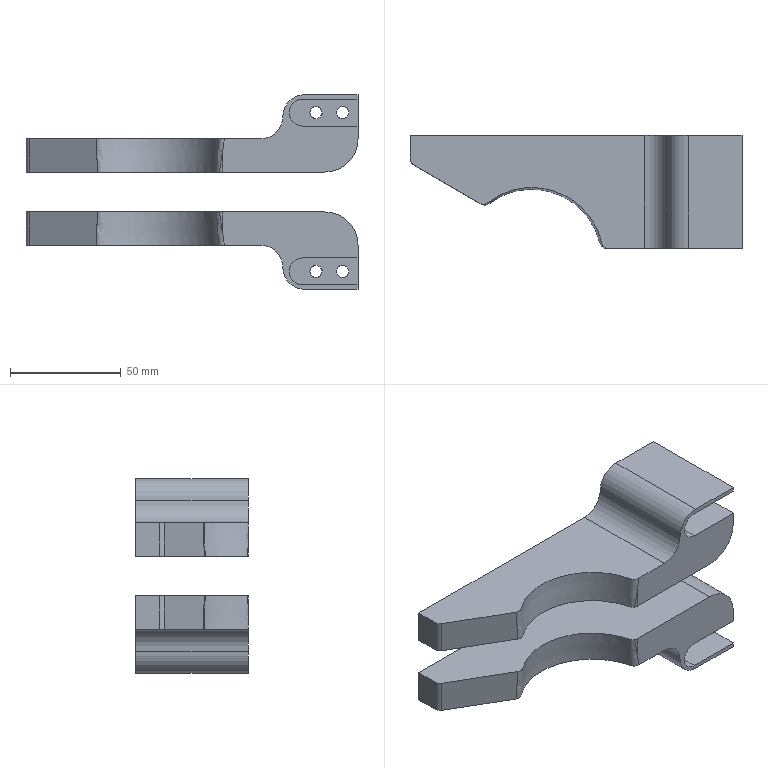NC program | NX | posted with a generic post | part box 150 x 51 x 88 mm
Lines 8852 to 9163 of 21230:
(ZLEVEL_PROFILE_COPY_COPY_COPY_1_COPY_COPY_COPY_COPY , TOOL : D12JING)
N17678 T11 M6
N17680 G54
N17682 G17 G0 G90 X-77.567 Y26.742 S9500 M3
N17684 G43 Z30. H11
N17686 Z-8.5
N17688 G94 G1 X-76.038 Y24.095 F1000.
N17690 G3 X-75. Y23.495 R1.199
N17692 G1 X60.005 F1200.
N17694 G2 X80.995 Y2.5 R20.995
N17696 G1 Y-17.5
N17698 G2 X75. Y-23.495 R5.995
N17700 G1 X51.
N17702 G2 X35.005 Y-7.5 R15.995
N17704 G3 X31. Y-3.495 R4.005
N17706 G1 X-75.
N17708 G2 X-80.995 Y2.5 R5.995
N17710 G1 Y17.5
N17712 G2 X-75. Y23.495 R5.995
N17714 G3 X-73.962 Y24.095 R1.199
N17716 G1 X-72.231 Y27.092
N17718 G0 X-77.567 Y26.742 Z-17.
N17720 G1 X-76.038 Y24.095 F1000.
N17722 G3 X-75. Y23.495 R1.199
N17724 G1 X60.005 F1200.
N17726 G2 X80.995 Y2.5 R20.995
N17728 G1 Y-17.5
N17730 G2 X75. Y-23.495 R5.995
N17732 G1 X51.
N17734 G2 X35.005 Y-7.5 R15.995
N17736 G3 X31. Y-3.495 R4.005
N17738 G1 X-75.
N17740 G2 X-80.995 Y2.5 R5.995
N17742 G1 Y17.5
N17744 G2 X-75. Y23.495 R5.995
N17746 G3 X-73.962 Y24.095 R1.199
N17748 G1 X-72.231 Y27.092
N17750 G0 X-77.567 Y26.742 Z-25.5
N17752 G1 X-76.038 Y24.095 F1000.
N17754 G3 X-75. Y23.495 R1.199
N17756 G1 X60.005 F1200.
N17758 G2 X80.995 Y2.5 R20.995
N17760 G1 Y-17.5
N17762 G2 X75. Y-23.495 R5.995
N17764 G1 X51.
N17766 G2 X35.005 Y-7.5 R15.995
N17768 G3 X31. Y-3.495 R4.005
N17770 G1 X-75.
N17772 G2 X-80.995 Y2.5 R5.995
N17774 G1 Y17.5
N17776 G2 X-75. Y23.495 R5.995
N17778 G3 X-73.962 Y24.095 R1.199
N17780 G1 X-72.231 Y27.092
N17782 G0 X-77.567 Y26.742 Z-34.
N17784 G1 X-76.038 Y24.095 F1000.
N17786 G3 X-75. Y23.495 R1.199
N17788 G1 X60.005 F1200.
N17790 G2 X80.995 Y2.5 R20.995
N17792 G1 Y-17.5
N17794 G2 X75. Y-23.495 R5.995
N17796 G1 X51.
N17798 G2 X35.005 Y-7.5 R15.995
N17800 G3 X31. Y-3.495 R4.005
N17802 G1 X-75.
N17804 G2 X-80.995 Y2.5 R5.995
N17806 G1 Y17.5
N17808 G2 X-75. Y23.495 R5.995
N17810 G3 X-73.962 Y24.095 R1.199
N17812 G1 X-72.231 Y27.092
N17814 G0 X-77.567 Y26.742 Z-42.5
N17816 G1 X-76.038 Y24.095 F1000.
N17818 G3 X-75. Y23.495 R1.199
N17820 G1 X60.005 F1200.
N17822 G2 X80.995 Y2.5 R20.995
N17824 G1 Y-17.5
N17826 G2 X75. Y-23.495 R5.995
N17828 G1 X51.
N17830 G2 X35.005 Y-7.5 R15.995
N17832 G3 X31. Y-3.495 R4.005
N17834 G1 X-75.
N17836 G2 X-80.995 Y2.5 R5.995
N17838 G1 Y17.5
N17840 G2 X-75. Y23.495 R5.995
N17842 G3 X-73.962 Y24.095 R1.199
N17844 G1 X-72.231 Y27.092
N17846 G0 X-77.567 Y26.742 Z-51.
N17848 G1 X-76.038 Y24.095 F1000.
N17850 G3 X-75. Y23.495 R1.199
N17852 G1 X60.005 F1200.
N17854 G2 X80.995 Y2.5 R20.995
N17856 G1 Y-17.5
N17858 G2 X75. Y-23.495 R5.995
N17860 G1 X51.
N17862 G2 X35.005 Y-7.5 R15.995
N17864 G3 X31. Y-3.495 R4.005
N17866 G1 X-75.
N17868 G2 X-80.995 Y2.5 R5.995
N17870 G1 Y17.5
N17872 G2 X-75. Y23.495 R5.995
N17874 G3 X-73.962 Y24.095 R1.199
N17876 G1 X-72.231 Y27.092
N17878 G0 Z30.
(ZLEVEL_PROFILE_COPY , TOOL : D12JING)
N17880 X81.455 Y-9.292
N17882 Z0.
N17884 G1 Z-0.95 F1650.
N17886 X80.966 Y-9.295
N17888 X74.609
N17890 X50.
N17892 G3 X49.895 Y-9.4 R0.105
N17894 X50. Y-9.505 R0.105
N17896 G1 X74.609
N17898 X80.966
N17900 X81.455 Y-9.507
N17902 G3 X81.755 Y-9.429 R0.6
N17904 G0 X81.455 Y-9.292
N17906 G1 Z-1.9
N17908 X80.966 Y-9.296
N17910 X74.609 Y-9.295
N17912 X50.
N17914 G3 X49.895 Y-9.4 R0.105
N17916 X50. Y-9.505 R0.105
N17918 G1 X74.609
N17920 X80.966 Y-9.504
N17922 X81.455 Y-9.507
N17924 G3 X81.755 Y-9.429 R0.6
N17926 G0 X81.455 Y-9.292
N17928 G1 Z-2.85
N17930 X80.966 Y-9.296
N17932 X74.609 Y-9.295
N17934 X50.
N17936 G3 X49.895 Y-9.4 R0.105
N17938 X50. Y-9.505 R0.105
N17940 G1 X74.609
N17942 X80.966 Y-9.504
N17944 X81.455 Y-9.507
N17946 G3 X81.755 Y-9.429 R0.6
N17948 G0 X81.455 Y-9.292
N17950 G1 Z-3.8
N17952 X80.966 Y-9.296
N17954 X75.098
N17956 X74.609 Y-9.295
N17958 X50.
N17960 G3 X49.895 Y-9.4 R0.105
N17962 X50. Y-9.505 R0.105
N17964 G1 X74.609
N17966 X75.098 Y-9.504
N17968 X80.966
N17970 X81.455 Y-9.507
N17972 G3 X81.755 Y-9.428 R0.6
N17974 G0 X81.455 Y-9.292
N17976 G1 Z-4.75
N17978 X80.966 Y-9.296
N17980 X75.098
N17982 X74.609 Y-9.295
N17984 X50.
N17986 G3 X49.895 Y-9.4 R0.105
N17988 X50. Y-9.505 R0.105
N17990 G1 X74.609
N17992 X75.098 Y-9.504
N17994 X80.966
N17996 X81.455 Y-9.507
N17998 G3 X81.755 Y-9.428 R0.6
N18000 G0 X81.455 Y-9.292
N18002 G1 Z-5.7
N18004 X80.966 Y-9.296
N18006 X75.098
N18008 X74.609 Y-9.295
N18010 X50.
N18012 G3 X49.895 Y-9.4 R0.105
N18014 X50. Y-9.505 R0.105
N18016 G1 X74.609
N18018 X75.098 Y-9.504
N18020 X80.966
N18022 X81.455 Y-9.507
N18024 G3 X81.755 Y-9.428 R0.6
N18026 G0 X81.455 Y-9.293
N18028 G1 Z-6.65
N18030 X80.966 Y-9.296
N18032 X75.098
N18034 X74.609 Y-9.295
N18036 X50.
N18038 G3 X49.895 Y-9.4 R0.105
N18040 X50. Y-9.505 R0.105
N18042 G1 X74.609
N18044 X75.098 Y-9.504
N18046 X80.966
N18048 X81.455 Y-9.507
N18050 G3 X81.755 Y-9.428 R0.6
N18052 G0 X81.455 Y-9.293
N18054 G1 Z-7.6
N18056 X80.966 Y-9.296
N18058 X75.098
N18060 X74.609 Y-9.295
N18062 X50.
N18064 G3 X49.895 Y-9.4 R0.105
N18066 X50. Y-9.505 R0.105
N18068 G1 X74.609
N18070 X75.098 Y-9.504
N18072 X80.966
N18074 X81.455 Y-9.507
N18076 G3 X81.755 Y-9.428 R0.6
N18078 G0 X81.455 Y-9.293
N18080 G1 Z-8.55
N18082 X80.966 Y-9.296
N18084 X75.098
N18086 X74.609 Y-9.295
N18088 X50.
N18090 G3 X49.895 Y-9.4 R0.105
N18092 X50. Y-9.505 R0.105
N18094 G1 X74.609
N18096 X75.098 Y-9.504
N18098 X80.966
N18100 X81.455 Y-9.507
N18102 G3 X81.755 Y-9.428 R0.6
N18104 G0 X81.455 Y-9.293
N18106 G1 Z-9.5
N18108 X80.966 Y-9.296
N18110 X75.098
N18112 X74.609 Y-9.295
N18114 X50.
N18116 G3 X49.895 Y-9.4 R0.105
N18118 X50. Y-9.505 R0.105
N18120 G1 X74.609
N18122 X75.098 Y-9.504
N18124 X80.966
N18126 X81.455 Y-9.506
N18128 G3 X81.755 Y-9.428 R0.6
N18130 G0 X81.455 Y-9.293
N18132 G1 Z-10.45
N18134 X80.966 Y-9.296
N18136 X75.098
N18138 X74.609 Y-9.295
N18140 X50.
N18142 G3 X49.895 Y-9.4 R0.105
N18144 X50. Y-9.505 R0.105
N18146 G1 X74.609
N18148 X75.098 Y-9.504
N18150 X80.966
N18152 X81.455 Y-9.506
N18154 G3 X81.755 Y-9.428 R0.6
N18156 G0 X81.455 Y-9.293
N18158 G1 Z-11.4
N18160 X80.966 Y-9.296
N18162 X75.098
N18164 X74.609 Y-9.295
N18166 X50.
N18168 G3 X49.895 Y-9.4 R0.105
N18170 X50. Y-9.505 R0.105
N18172 G1 X74.609
N18174 X75.098 Y-9.504
N18176 X80.966
N18178 X81.455 Y-9.506
N18180 G3 X81.755 Y-9.427 R0.6
N18182 G0 X81.455 Y-9.293
N18184 G1 Z-12.35
N18186 X80.966 Y-9.297
N18188 X75.098
N18190 X74.609 Y-9.295
N18192 X50.
N18194 G3 X49.895 Y-9.4 R0.105
N18196 X50. Y-9.505 R0.105
N18198 G1 X74.609
N18200 X75.098 Y-9.503
N18202 X80.966
N18204 X81.455 Y-9.506
N18206 G3 X81.755 Y-9.427 R0.6
N18208 G0 X81.455 Y-9.293
N18210 G1 Z-13.3
N18212 X80.966 Y-9.297
N18214 X75.098
N18216 X74.609 Y-9.295
N18218 X50.
N18220 G3 X49.895 Y-9.4 R0.105
N18222 X50. Y-9.505 R0.105
N18224 G1 X74.609
N18226 X75.098 Y-9.503
N18228 X80.966
N18230 X81.455 Y-9.506
N18232 G3 X81.755 Y-9.427 R0.6
N18234 G0 X81.455 Y-9.293
N18236 G1 Z-14.25
N18238 X80.966 Y-9.297
N18240 X75.098
N18242 X74.609 Y-9.295
N18244 X50.
N18246 G3 X49.895 Y-9.4 R0.105
N18248 X50. Y-9.505 R0.105
N18250 G1 X74.609
N18252 X75.098 Y-9.503
N18254 X80.966
N18256 X81.455 Y-9.506
N18258 G3 X81.755 Y-9.427 R0.6
N18260 G0 X81.455 Y-9.293
N18262 G1 Z-15.2
N18264 X80.966 Y-9.297
N18266 X75.098
N18268 X74.609 Y-9.295
N18270 X50.
N18272 G3 X49.895 Y-9.4 R0.105
N18274 X50. Y-9.505 R0.105
N18276 G1 X74.609
N18278 X75.098 Y-9.503
N18280 X80.966
N18282 X81.455 Y-9.506
N18284 G3 X81.755 Y-9.427 R0.6
N18286 G0 Z30.
N18288 M5